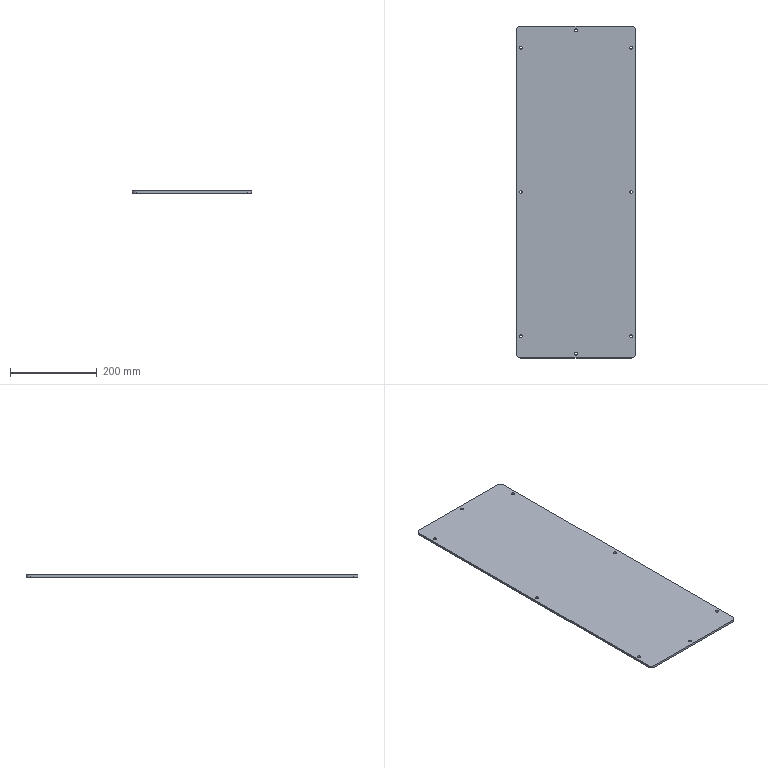Part | STEP file | 1 solid | 26 faces | box 274 x 764 x 5 mm | volume 1044923 mm3 | cylinder 20 | plane 6 | commonest cylinder face diameters 6.5 x16 20 x4